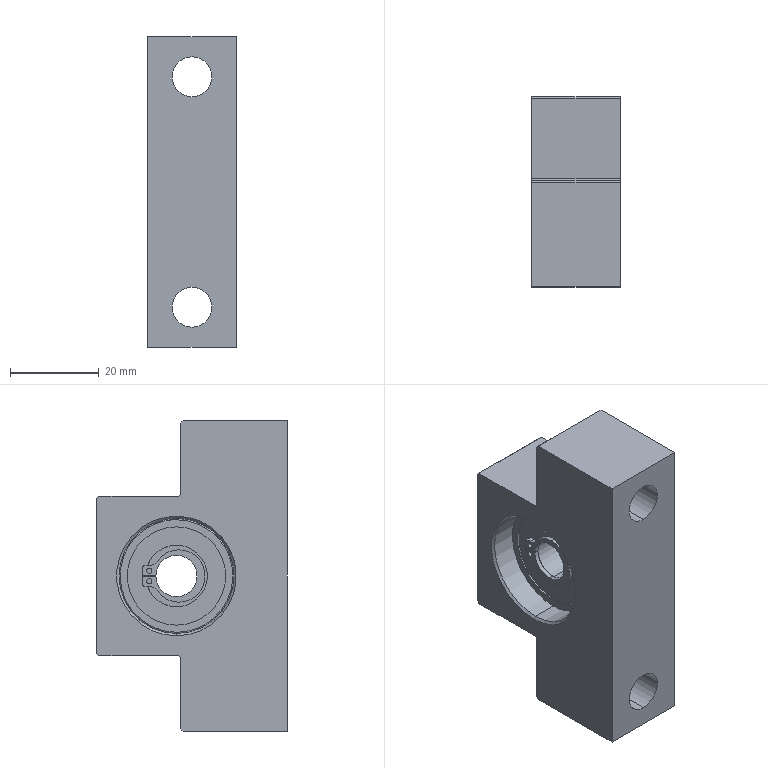Part | NX | features BREP 1 | 1 solid | 79 faces | box 20 x 43 x 70 mm | volume 37093 mm3 | plane 35 | cylinder 32 | torus 8 | cone 4 | commonest cylinder face diameters 1.2 x4 9 x4 13.9 x4 22.2 x4 26 x4 9.3 x3